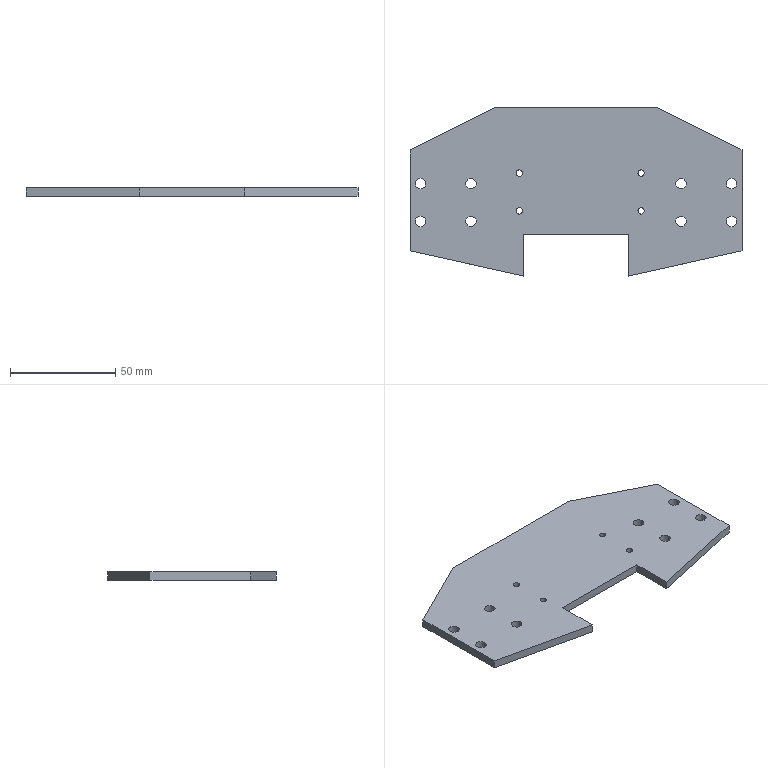Part | STEP file | Sliding plate | 1 solid | 36 faces | box 158 x 80 x 4 mm | volume 40027 mm3 | cylinder 24 | plane 12 | commonest cylinder face diameters 5 x16 3 x8